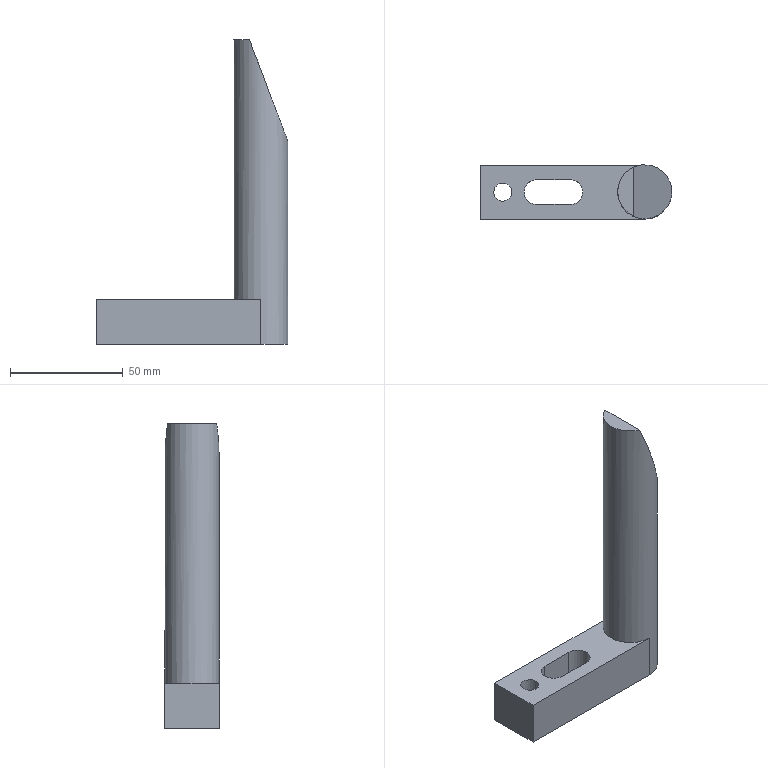Part | NX | features MAIN_BODY 2 | 1 solid | 13 faces | box 85 x 24 x 135 mm | volume 78557 mm3 | plane 9 | cylinder 4 | commonest cylinder face diameters 11 x2 8 x1 24 x1
STEP:
#1=CARTESIAN_POINT('',(-748.,505.,-120.));
#2=VERTEX_POINT('',#1);
#3=CARTESIAN_POINT('',(-748.,481.,-120.));
#4=VERTEX_POINT('',#3);
#5=CARTESIAN_POINT('',(-748.,493.,-120.));
#6=DIRECTION('',(0.,0.,-1.));
#7=DIRECTION('',(1.,0.,0.));
#8=AXIS2_PLACEMENT_3D('',#5,#6,#7);
#9=CIRCLE('',#8,12.);
#10=EDGE_CURVE('',#2,#4,#9,.T.);
#11=ORIENTED_EDGE('',*,*,#10,.F.);
#12=CARTESIAN_POINT('',(-748.,505.,-100.));
#13=VERTEX_POINT('',#12);
#14=CARTESIAN_POINT('',(-748.,505.,-70.));
#15=DIRECTION('',(0.,0.,-1.));
#16=VECTOR('',#15,1000.);
#17=LINE('',#14,#16);
#18=EDGE_CURVE('',#13,#2,#17,.T.);
#19=ORIENTED_EDGE('',*,*,#18,.F.);
#20=CARTESIAN_POINT('',(-748.,481.,-100.));
#21=VERTEX_POINT('',#20);
#22=CARTESIAN_POINT('',(-748.,493.,-100.));
#23=DIRECTION('',(0.,0.,-1.));
#24=DIRECTION('',(1.,0.,0.));
#25=AXIS2_PLACEMENT_3D('',#22,#23,#24);
#26=CIRCLE('',#25,12.);
#27=EDGE_CURVE('',#13,#21,#26,.F.);
#28=ORIENTED_EDGE('',*,*,#27,.T.);
#29=CARTESIAN_POINT('',(-748.,481.,-70.));
#30=DIRECTION('',(0.,0.,-1.));
#31=VECTOR('',#30,1000.);
#32=LINE('',#29,#31);
#33=EDGE_CURVE('',#21,#4,#32,.T.);
#34=ORIENTED_EDGE('',*,*,#33,.T.);
#35=EDGE_LOOP('',(#11,#19,#28,#34));
#36=FACE_BOUND('',#35,.T.);
#37=CARTESIAN_POINT('',(-753.,503.909,15.));
#38=VERTEX_POINT('',#37);
#39=CARTESIAN_POINT('',(-753.,482.091,15.));
#40=VERTEX_POINT('',#39);
#41=CARTESIAN_POINT('',(-748.,493.,1.765));
#42=DIRECTION('',(-0.9355,0.,-0.3534));
#43=DIRECTION('',(0.3534,0.,-0.9355));
#44=AXIS2_PLACEMENT_3D('',#41,#42,#43);
#45=ELLIPSE('',#44,33.956,12.);
#46=EDGE_CURVE('',#38,#40,#45,.T.);
#47=ORIENTED_EDGE('',*,*,#46,.T.);
#48=CARTESIAN_POINT('',(-748.,493.,15.));
#49=DIRECTION('',(0.,0.,-1.));
#50=DIRECTION('',(0.,1.,0.));
#51=AXIS2_PLACEMENT_3D('',#48,#49,#50);
#52=CIRCLE('',#51,12.);
#53=EDGE_CURVE('',#40,#38,#52,.T.);
#54=ORIENTED_EDGE('',*,*,#53,.T.);
#55=EDGE_LOOP('',(#47,#54));
#56=FACE_BOUND('',#55,.T.);
#57=CARTESIAN_POINT('',(-748.,493.,10.));
#58=DIRECTION('',(0.,0.,-1.));
#59=DIRECTION('',(0.,-1.,0.));
#60=AXIS2_PLACEMENT_3D('',#57,#58,#59);
#61=CYLINDRICAL_SURFACE('',#60,12.);
#62=ADVANCED_FACE('',(#36,#56),#61,.T.);
#63=ORIENTED_EDGE('',*,*,#53,.F.);
#64=CARTESIAN_POINT('',(-753.,493.,15.));
#65=DIRECTION('',(0.,-1.,0.));
#66=VECTOR('',#65,1000.);
#67=LINE('',#64,#66);
#68=EDGE_CURVE('',#38,#40,#67,.T.);
#69=ORIENTED_EDGE('',*,*,#68,.F.);
#70=EDGE_LOOP('',(#63,#69));
#71=FACE_BOUND('',#70,.T.);
#72=CARTESIAN_POINT('',(-748.,493.,15.));
#73=DIRECTION('',(0.,0.,1.));
#74=DIRECTION('',(0.,1.,0.));
#75=AXIS2_PLACEMENT_3D('',#72,#73,#74);
#76=PLANE('',#75);
#77=ADVANCED_FACE('',(#71),#76,.T.);
#78=CARTESIAN_POINT('',(-807.,493.,-100.));
#79=VERTEX_POINT('',#78);
#80=CARTESIAN_POINT('',(-811.,493.,-100.));
#81=DIRECTION('',(0.,0.,-1.));
#82=DIRECTION('',(1.,0.,0.));
#83=AXIS2_PLACEMENT_3D('',#80,#81,#82);
#84=CIRCLE('',#83,4.);
#85=EDGE_CURVE('',#79,#79,#84,.F.);
#86=ORIENTED_EDGE('',*,*,#85,.F.);
#87=EDGE_LOOP('',(#86));
#88=FACE_BOUND('',#87,.T.);
#89=CARTESIAN_POINT('',(-796.,487.5,-100.));
#90=VERTEX_POINT('',#89);
#91=CARTESIAN_POINT('',(-781.,487.5,-100.));
#92=VERTEX_POINT('',#91);
#93=CARTESIAN_POINT('',(-776.,487.5,-100.));
#94=DIRECTION('',(1.,0.,0.));
#95=VECTOR('',#94,1000.);
#96=LINE('',#93,#95);
#97=EDGE_CURVE('',#90,#92,#96,.T.);
#98=ORIENTED_EDGE('',*,*,#97,.F.);
#99=CARTESIAN_POINT('',(-796.,498.5,-100.));
#100=VERTEX_POINT('',#99);
#101=CARTESIAN_POINT('',(-796.,493.,-100.));
#102=DIRECTION('',(0.,0.,-1.));
#103=DIRECTION('',(1.,0.,0.));
#104=AXIS2_PLACEMENT_3D('',#101,#102,#103);
#105=CIRCLE('',#104,5.5);
#106=EDGE_CURVE('',#90,#100,#105,.T.);
#107=ORIENTED_EDGE('',*,*,#106,.T.);
#108=CARTESIAN_POINT('',(-781.,498.5,-100.));
#109=VERTEX_POINT('',#108);
#110=CARTESIAN_POINT('',(-776.,498.5,-100.));
#111=DIRECTION('',(1.,0.,0.));
#112=VECTOR('',#111,1000.);
#113=LINE('',#110,#112);
#114=EDGE_CURVE('',#100,#109,#113,.T.);
#115=ORIENTED_EDGE('',*,*,#114,.T.);
#116=CARTESIAN_POINT('',(-781.,493.,-100.));
#117=DIRECTION('',(0.,0.,-1.));
#118=DIRECTION('',(1.,0.,0.));
#119=AXIS2_PLACEMENT_3D('',#116,#117,#118);
#120=CIRCLE('',#119,5.5);
#121=EDGE_CURVE('',#109,#92,#120,.T.);
#122=ORIENTED_EDGE('',*,*,#121,.T.);
#123=EDGE_LOOP('',(#98,#107,#115,#122));
#124=FACE_BOUND('',#123,.T.);
#125=CARTESIAN_POINT('',(-821.,505.,-100.));
#126=VERTEX_POINT('',#125);
#127=CARTESIAN_POINT('',(-816.,505.,-100.));
#128=DIRECTION('',(1.,0.,0.));
#129=VECTOR('',#128,1000.);
#130=LINE('',#127,#129);
#131=EDGE_CURVE('',#126,#13,#130,.T.);
#132=ORIENTED_EDGE('',*,*,#131,.F.);
#133=CARTESIAN_POINT('',(-821.,481.,-100.));
#134=VERTEX_POINT('',#133);
#135=CARTESIAN_POINT('',(-821.,481.,-100.));
#136=DIRECTION('',(0.,1.,0.));
#137=VECTOR('',#136,1000.);
#138=LINE('',#135,#137);
#139=EDGE_CURVE('',#134,#126,#138,.T.);
#140=ORIENTED_EDGE('',*,*,#139,.F.);
#141=CARTESIAN_POINT('',(-728.,481.,-100.));
#142=DIRECTION('',(-1.,0.,0.));
#143=VECTOR('',#142,1000.);
#144=LINE('',#141,#143);
#145=EDGE_CURVE('',#21,#134,#144,.T.);
#146=ORIENTED_EDGE('',*,*,#145,.F.);
#147=ORIENTED_EDGE('',*,*,#27,.F.);
#148=EDGE_LOOP('',(#132,#140,#146,#147));
#149=FACE_BOUND('',#148,.T.);
#150=CARTESIAN_POINT('',(-728.,481.,-100.));
#151=DIRECTION('',(0.,0.,1.));
#152=DIRECTION('',(0.,1.,0.));
#153=AXIS2_PLACEMENT_3D('',#150,#151,#152);
#154=PLANE('',#153);
#155=ADVANCED_FACE('',(#88,#124,#149),#154,.T.);
#156=CARTESIAN_POINT('',(-821.,481.,-120.));
#157=VERTEX_POINT('',#156);
#158=CARTESIAN_POINT('',(-728.,481.,-120.));
#159=DIRECTION('',(-1.,0.,0.));
#160=VECTOR('',#159,1000.);
#161=LINE('',#158,#160);
#162=EDGE_CURVE('',#4,#157,#161,.T.);
#163=ORIENTED_EDGE('',*,*,#162,.F.);
#164=ORIENTED_EDGE('',*,*,#33,.F.);
#165=ORIENTED_EDGE('',*,*,#145,.T.);
#166=CARTESIAN_POINT('',(-821.,481.,-70.));
#167=DIRECTION('',(0.,0.,-1.));
#168=VECTOR('',#167,1000.);
#169=LINE('',#166,#168);
#170=EDGE_CURVE('',#134,#157,#169,.T.);
#171=ORIENTED_EDGE('',*,*,#170,.T.);
#172=EDGE_LOOP('',(#163,#164,#165,#171));
#173=FACE_BOUND('',#172,.T.);
#174=CARTESIAN_POINT('',(-748.,481.,-70.));
#175=DIRECTION('',(0.,1.,0.));
#176=DIRECTION('',(1.,0.,0.));
#177=AXIS2_PLACEMENT_3D('',#174,#175,#176);
#178=PLANE('',#177);
#179=ADVANCED_FACE('',(#173),#178,.F.);
#180=CARTESIAN_POINT('',(-821.,505.,-120.));
#181=VERTEX_POINT('',#180);
#182=CARTESIAN_POINT('',(-821.,481.,-120.));
#183=DIRECTION('',(0.,1.,0.));
#184=VECTOR('',#183,1000.);
#185=LINE('',#182,#184);
#186=EDGE_CURVE('',#157,#181,#185,.T.);
#187=ORIENTED_EDGE('',*,*,#186,.F.);
#188=ORIENTED_EDGE('',*,*,#170,.F.);
#189=ORIENTED_EDGE('',*,*,#139,.T.);
#190=CARTESIAN_POINT('',(-821.,505.,-70.));
#191=DIRECTION('',(0.,0.,-1.));
#192=VECTOR('',#191,1000.);
#193=LINE('',#190,#192);
#194=EDGE_CURVE('',#126,#181,#193,.T.);
#195=ORIENTED_EDGE('',*,*,#194,.T.);
#196=EDGE_LOOP('',(#187,#188,#189,#195));
#197=FACE_BOUND('',#196,.T.);
#198=CARTESIAN_POINT('',(-821.,481.,-70.));
#199=DIRECTION('',(1.,0.,0.));
#200=DIRECTION('',(0.,0.,1.));
#201=AXIS2_PLACEMENT_3D('',#198,#199,#200);
#202=PLANE('',#201);
#203=ADVANCED_FACE('',(#197),#202,.F.);
#204=CARTESIAN_POINT('',(-816.,505.,-120.));
#205=DIRECTION('',(1.,0.,0.));
#206=VECTOR('',#205,1000.);
#207=LINE('',#204,#206);
#208=EDGE_CURVE('',#181,#2,#207,.T.);
#209=ORIENTED_EDGE('',*,*,#208,.F.);
#210=ORIENTED_EDGE('',*,*,#194,.F.);
#211=ORIENTED_EDGE('',*,*,#131,.T.);
#212=ORIENTED_EDGE('',*,*,#18,.T.);
#213=EDGE_LOOP('',(#209,#210,#211,#212));
#214=FACE_BOUND('',#213,.T.);
#215=CARTESIAN_POINT('',(-836.,505.,-70.));
#216=DIRECTION('',(0.,-1.,0.));
#217=DIRECTION('',(-1.,0.,0.));
#218=AXIS2_PLACEMENT_3D('',#215,#216,#217);
#219=PLANE('',#218);
#220=ADVANCED_FACE('',(#214),#219,.F.);
#221=CARTESIAN_POINT('',(-807.,493.,-120.));
#222=VERTEX_POINT('',#221);
#223=CARTESIAN_POINT('',(-811.,493.,-120.));
#224=DIRECTION('',(0.,0.,-1.));
#225=DIRECTION('',(1.,0.,0.));
#226=AXIS2_PLACEMENT_3D('',#223,#224,#225);
#227=CIRCLE('',#226,4.);
#228=EDGE_CURVE('',#222,#222,#227,.F.);
#229=ORIENTED_EDGE('',*,*,#228,.T.);
#230=EDGE_LOOP('',(#229));
#231=FACE_BOUND('',#230,.T.);
#232=CARTESIAN_POINT('',(-781.,498.5,-120.));
#233=VERTEX_POINT('',#232);
#234=CARTESIAN_POINT('',(-781.,487.5,-120.));
#235=VERTEX_POINT('',#234);
#236=CARTESIAN_POINT('',(-781.,493.,-120.));
#237=DIRECTION('',(0.,0.,-1.));
#238=DIRECTION('',(1.,0.,0.));
#239=AXIS2_PLACEMENT_3D('',#236,#237,#238);
#240=CIRCLE('',#239,5.5);
#241=EDGE_CURVE('',#233,#235,#240,.T.);
#242=ORIENTED_EDGE('',*,*,#241,.F.);
#243=CARTESIAN_POINT('',(-796.,498.5,-120.));
#244=VERTEX_POINT('',#243);
#245=CARTESIAN_POINT('',(-791.,498.5,-120.));
#246=DIRECTION('',(1.,0.,0.));
#247=VECTOR('',#246,1000.);
#248=LINE('',#245,#247);
#249=EDGE_CURVE('',#244,#233,#248,.T.);
#250=ORIENTED_EDGE('',*,*,#249,.F.);
#251=CARTESIAN_POINT('',(-796.,487.5,-120.));
#252=VERTEX_POINT('',#251);
#253=CARTESIAN_POINT('',(-796.,493.,-120.));
#254=DIRECTION('',(0.,0.,-1.));
#255=DIRECTION('',(1.,0.,0.));
#256=AXIS2_PLACEMENT_3D('',#253,#254,#255);
#257=CIRCLE('',#256,5.5);
#258=EDGE_CURVE('',#252,#244,#257,.T.);
#259=ORIENTED_EDGE('',*,*,#258,.F.);
#260=CARTESIAN_POINT('',(-791.,487.5,-120.));
#261=DIRECTION('',(1.,0.,0.));
#262=VECTOR('',#261,1000.);
#263=LINE('',#260,#262);
#264=EDGE_CURVE('',#252,#235,#263,.T.);
#265=ORIENTED_EDGE('',*,*,#264,.T.);
#266=EDGE_LOOP('',(#242,#250,#259,#265));
#267=FACE_BOUND('',#266,.T.);
#268=ORIENTED_EDGE('',*,*,#162,.T.);
#269=ORIENTED_EDGE('',*,*,#186,.T.);
#270=ORIENTED_EDGE('',*,*,#208,.T.);
#271=ORIENTED_EDGE('',*,*,#10,.T.);
#272=EDGE_LOOP('',(#268,#269,#270,#271));
#273=FACE_BOUND('',#272,.T.);
#274=CARTESIAN_POINT('',(-728.,481.,-120.));
#275=DIRECTION('',(0.,0.,1.));
#276=DIRECTION('',(0.,1.,0.));
#277=AXIS2_PLACEMENT_3D('',#274,#275,#276);
#278=PLANE('',#277);
#279=ADVANCED_FACE('',(#231,#267,#273),#278,.F.);
#280=ORIENTED_EDGE('',*,*,#68,.T.);
#281=ORIENTED_EDGE('',*,*,#46,.F.);
#282=EDGE_LOOP('',(#280,#281));
#283=FACE_BOUND('',#282,.T.);
#284=CARTESIAN_POINT('',(-753.,421.5,15.));
#285=DIRECTION('',(0.9355,0.,0.3534));
#286=DIRECTION('',(-0.3534,0.,0.9355));
#287=AXIS2_PLACEMENT_3D('',#284,#285,#286);
#288=PLANE('',#287);
#289=ADVANCED_FACE('',(#283),#288,.T.);
#290=ORIENTED_EDGE('',*,*,#97,.T.);
#291=CARTESIAN_POINT('',(-781.,487.5,-70.));
#292=DIRECTION('',(0.,0.,1.));
#293=VECTOR('',#292,1000.);
#294=LINE('',#291,#293);
#295=EDGE_CURVE('',#235,#92,#294,.T.);
#296=ORIENTED_EDGE('',*,*,#295,.F.);
#297=ORIENTED_EDGE('',*,*,#264,.F.);
#298=CARTESIAN_POINT('',(-796.,487.5,-70.));
#299=DIRECTION('',(0.,0.,1.));
#300=VECTOR('',#299,1000.);
#301=LINE('',#298,#300);
#302=EDGE_CURVE('',#252,#90,#301,.T.);
#303=ORIENTED_EDGE('',*,*,#302,.T.);
#304=EDGE_LOOP('',(#290,#296,#297,#303));
#305=FACE_BOUND('',#304,.T.);
#306=CARTESIAN_POINT('',(-796.,487.5,-70.));
#307=DIRECTION('',(0.,-1.,0.));
#308=DIRECTION('',(0.,0.,1.));
#309=AXIS2_PLACEMENT_3D('',#306,#307,#308);
#310=PLANE('',#309);
#311=ADVANCED_FACE('',(#305),#310,.F.);
#312=ORIENTED_EDGE('',*,*,#106,.F.);
#313=ORIENTED_EDGE('',*,*,#302,.F.);
#314=ORIENTED_EDGE('',*,*,#258,.T.);
#315=CARTESIAN_POINT('',(-796.,498.5,-70.));
#316=DIRECTION('',(0.,0.,1.));
#317=VECTOR('',#316,1000.);
#318=LINE('',#315,#317);
#319=EDGE_CURVE('',#244,#100,#318,.T.);
#320=ORIENTED_EDGE('',*,*,#319,.T.);
#321=EDGE_LOOP('',(#312,#313,#314,#320));
#322=FACE_BOUND('',#321,.T.);
#323=CARTESIAN_POINT('',(-796.,493.,-70.));
#324=DIRECTION('',(0.,0.,1.));
#325=DIRECTION('',(0.,1.,0.));
#326=AXIS2_PLACEMENT_3D('',#323,#324,#325);
#327=CYLINDRICAL_SURFACE('',#326,5.5);
#328=ADVANCED_FACE('',(#322),#327,.F.);
#329=ORIENTED_EDGE('',*,*,#114,.F.);
#330=ORIENTED_EDGE('',*,*,#319,.F.);
#331=ORIENTED_EDGE('',*,*,#249,.T.);
#332=CARTESIAN_POINT('',(-781.,498.5,-70.));
#333=DIRECTION('',(0.,0.,1.));
#334=VECTOR('',#333,1000.);
#335=LINE('',#332,#334);
#336=EDGE_CURVE('',#233,#109,#335,.T.);
#337=ORIENTED_EDGE('',*,*,#336,.T.);
#338=EDGE_LOOP('',(#329,#330,#331,#337));
#339=FACE_BOUND('',#338,.T.);
#340=CARTESIAN_POINT('',(-796.,498.5,-70.));
#341=DIRECTION('',(0.,1.,0.));
#342=DIRECTION('',(0.,0.,-1.));
#343=AXIS2_PLACEMENT_3D('',#340,#341,#342);
#344=PLANE('',#343);
#345=ADVANCED_FACE('',(#339),#344,.F.);
#346=ORIENTED_EDGE('',*,*,#121,.F.);
#347=ORIENTED_EDGE('',*,*,#336,.F.);
#348=ORIENTED_EDGE('',*,*,#241,.T.);
#349=ORIENTED_EDGE('',*,*,#295,.T.);
#350=EDGE_LOOP('',(#346,#347,#348,#349));
#351=FACE_BOUND('',#350,.T.);
#352=CARTESIAN_POINT('',(-781.,493.,-70.));
#353=DIRECTION('',(0.,0.,1.));
#354=DIRECTION('',(0.,1.,0.));
#355=AXIS2_PLACEMENT_3D('',#352,#353,#354);
#356=CYLINDRICAL_SURFACE('',#355,5.5);
#357=ADVANCED_FACE('',(#351),#356,.F.);
#358=ORIENTED_EDGE('',*,*,#228,.F.);
#359=EDGE_LOOP('',(#358));
#360=FACE_BOUND('',#359,.T.);
#361=ORIENTED_EDGE('',*,*,#85,.T.);
#362=EDGE_LOOP('',(#361));
#363=FACE_BOUND('',#362,.T.);
#364=CARTESIAN_POINT('',(-811.,493.,-70.));
#365=DIRECTION('',(0.,0.,-1.));
#366=DIRECTION('',(0.,-1.,0.));
#367=AXIS2_PLACEMENT_3D('',#364,#365,#366);
#368=CYLINDRICAL_SURFACE('',#367,4.);
#369=ADVANCED_FACE('',(#360,#363),#368,.F.);
#370=CLOSED_SHELL('',(#62,#77,#155,#179,#203,#220,#279,#289,#311,#328,#345,#357,#369));
#371=MANIFOLD_SOLID_BREP('',#370);
#372=(LENGTH_UNIT()NAMED_UNIT(*)SI_UNIT(.MILLI.,.METRE.));
#373=UNCERTAINTY_MEASURE_WITH_UNIT(LENGTH_MEASURE(0.00001),#372,'','');
#374=(NAMED_UNIT(*)PLANE_ANGLE_UNIT()SI_UNIT($,.RADIAN.));
#375=(NAMED_UNIT(*)SI_UNIT($,.STERADIAN.)SOLID_ANGLE_UNIT());
#376=(GEOMETRIC_REPRESENTATION_CONTEXT(3)GLOBAL_UNCERTAINTY_ASSIGNED_CONTEXT((#373))GLOBAL_UNIT_ASSIGNED_CONTEXT((#372,#374,#375))REPRESENTATION_CONTEXT('',''));
#377=ADVANCED_BREP_SHAPE_REPRESENTATION('',(#371),#376);